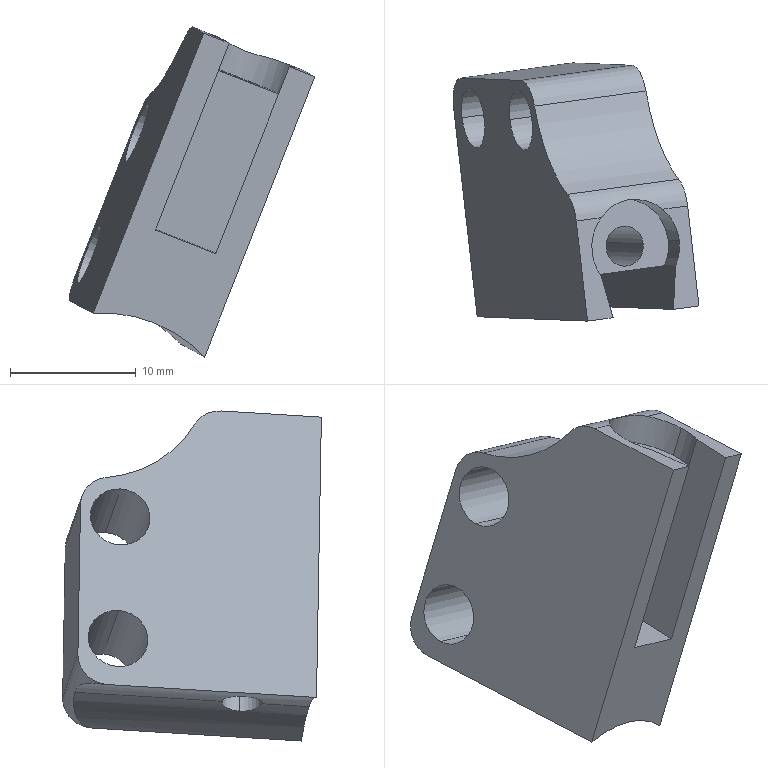Part | SolidWorks | features SplitBody 1 | 1 solid | 26 faces | box 19.582 x 20.608 x 26.296 mm | volume 2916 mm3 | cylinder 15 | plane 11 | commonest cylinder face diameters 4.8 x7 7.52 x3 3.2 x2 22.4 x2 19.2 x1
STEP:
#1=CARTESIAN_POINT('',(550.829,303.4,-344.866));
#2=VERTEX_POINT('',#1);
#3=CARTESIAN_POINT('',(555.434,305.978,-345.474));
#4=VERTEX_POINT('',#3);
#5=CARTESIAN_POINT('',(550.829,303.4,-344.866));
#6=CARTESIAN_POINT('',(550.801,303.644,-344.851));
#7=CARTESIAN_POINT('',(550.865,303.886,-344.83));
#8=CARTESIAN_POINT('',(551.105,304.312,-344.791));
#9=CARTESIAN_POINT('',(551.273,304.49,-344.775));
#10=CARTESIAN_POINT('',(551.646,304.799,-344.757));
#11=CARTESIAN_POINT('',(551.85,304.928,-344.755));
#12=CARTESIAN_POINT('',(552.277,305.154,-344.769));
#13=CARTESIAN_POINT('',(552.499,305.251,-344.784));
#14=CARTESIAN_POINT('',(553.17,305.506,-344.854));
#15=CARTESIAN_POINT('',(553.626,305.632,-344.933));
#16=CARTESIAN_POINT('',(554.544,305.84,-345.158));
#17=CARTESIAN_POINT('',(554.994,305.918,-345.302));
#18=CARTESIAN_POINT('',(555.434,305.978,-345.474));
#19=B_SPLINE_CURVE_WITH_KNOTS('',3,(#5,#6,#7,#8,#9,#10,#11,#12,#13,#14,#15,#16,#17,#18),.UNSPECIFIED.,.F.,.F.,(4,2,2,2,2,2,4),(0.,0.0007263,0.001453,0.002179,0.002905,0.004358,0.00581),.UNSPECIFIED.);
#20=EDGE_CURVE('',#2,#4,#19,.T.);
#21=ORIENTED_EDGE('',*,*,#20,.T.);
#22=CARTESIAN_POINT('',(556.757,294.247,-346.199));
#23=VERTEX_POINT('',#22);
#24=CARTESIAN_POINT('',(555.39,306.37,-345.45));
#25=DIRECTION('',(0.1119,-0.9918,-0.06132));
#26=VECTOR('',#25,1000.);
#27=LINE('',#24,#26);
#28=EDGE_CURVE('',#4,#23,#27,.T.);
#29=ORIENTED_EDGE('',*,*,#28,.T.);
#30=CARTESIAN_POINT('',(555.416,292.46,-345.826));
#31=VERTEX_POINT('',#30);
#32=CARTESIAN_POINT('',(555.416,292.46,-345.826));
#33=CARTESIAN_POINT('',(555.405,292.565,-345.819));
#34=CARTESIAN_POINT('',(555.403,292.669,-345.815));
#35=CARTESIAN_POINT('',(555.42,292.877,-345.812));
#36=CARTESIAN_POINT('',(555.439,292.982,-345.813));
#37=CARTESIAN_POINT('',(555.495,293.184,-345.82));
#38=CARTESIAN_POINT('',(555.533,293.282,-345.826));
#39=CARTESIAN_POINT('',(555.626,293.468,-345.845));
#40=CARTESIAN_POINT('',(555.682,293.558,-345.857));
#41=CARTESIAN_POINT('',(555.869,293.805,-345.903));
#42=CARTESIAN_POINT('',(556.026,293.946,-345.946));
#43=CARTESIAN_POINT('',(556.372,294.153,-346.056));
#44=CARTESIAN_POINT('',(556.564,294.221,-346.124));
#45=CARTESIAN_POINT('',(556.757,294.247,-346.199));
#46=B_SPLINE_CURVE_WITH_KNOTS('',3,(#32,#33,#34,#35,#36,#37,#38,#39,#40,#41,#42,#43,#44,#45),.UNSPECIFIED.,.F.,.F.,(4,2,2,2,2,2,4),(0.,0.0003131,0.0006262,0.0009394,0.001252,0.001879,0.002505),.UNSPECIFIED.);
#47=EDGE_CURVE('',#31,#23,#46,.T.);
#48=ORIENTED_EDGE('',*,*,#47,.F.);
#49=CARTESIAN_POINT('',(557.115,291.073,-346.396));
#50=VERTEX_POINT('',#49);
#51=CARTESIAN_POINT('',(557.115,291.073,-346.396));
#52=CARTESIAN_POINT('',(557.018,291.06,-346.357));
#53=CARTESIAN_POINT('',(556.92,291.057,-346.32));
#54=CARTESIAN_POINT('',(556.724,291.072,-346.249));
#55=CARTESIAN_POINT('',(556.625,291.09,-346.215));
#56=CARTESIAN_POINT('',(556.434,291.145,-346.15));
#57=CARTESIAN_POINT('',(556.341,291.182,-346.119));
#58=CARTESIAN_POINT('',(556.163,291.275,-346.062));
#59=CARTESIAN_POINT('',(556.076,291.332,-346.035));
#60=CARTESIAN_POINT('',(555.839,291.523,-345.963));
#61=CARTESIAN_POINT('',(555.704,291.685,-345.923));
#62=CARTESIAN_POINT('',(555.505,292.047,-345.861));
#63=CARTESIAN_POINT('',(555.44,292.25,-345.839));
#64=CARTESIAN_POINT('',(555.416,292.46,-345.826));
#65=B_SPLINE_CURVE_WITH_KNOTS('',3,(#51,#52,#53,#54,#55,#56,#57,#58,#59,#60,#61,#62,#63,#64),.UNSPECIFIED.,.F.,.F.,(4,2,2,2,2,2,4),(0.007514,0.007826,0.008139,0.008452,0.008765,0.009391,0.01002),.UNSPECIFIED.);
#66=EDGE_CURVE('',#50,#31,#65,.T.);
#67=ORIENTED_EDGE('',*,*,#66,.F.);
#68=CARTESIAN_POINT('',(557.538,287.327,-346.627));
#69=VERTEX_POINT('',#68);
#70=CARTESIAN_POINT('',(555.39,306.37,-345.45));
#71=DIRECTION('',(0.1119,-0.9918,-0.06132));
#72=VECTOR('',#71,1000.);
#73=LINE('',#70,#72);
#74=EDGE_CURVE('',#50,#69,#73,.T.);
#75=ORIENTED_EDGE('',*,*,#74,.T.);
#76=CARTESIAN_POINT('',(552.708,286.737,-345.897));
#77=VERTEX_POINT('',#76);
#78=CARTESIAN_POINT('',(553.434,287.509,-357.046));
#79=DIRECTION('',(0.1119,-0.9918,-0.06132));
#80=DIRECTION('',(0.3665,-0.01618,0.9303));
#81=AXIS2_PLACEMENT_3D('',#78,#79,#80);
#82=CIRCLE('',#81,11.2);
#83=EDGE_CURVE('',#69,#77,#82,.T.);
#84=ORIENTED_EDGE('',*,*,#83,.T.);
#85=CARTESIAN_POINT('',(552.708,286.737,-345.897));
#86=DIRECTION('',(0.1119,-0.9918,-0.06132));
#87=VECTOR('',#86,1000.);
#88=LINE('',#85,#87);
#89=EDGE_CURVE('',#2,#77,#88,.T.);
#90=ORIENTED_EDGE('',*,*,#89,.F.);
#91=EDGE_LOOP('',(#21,#29,#48,#67,#75,#84,#90));
#92=FACE_OUTER_BOUND('',#91,.T.);
#93=CARTESIAN_POINT('',(551.286,306.552,-355.869));
#94=DIRECTION('',(0.1119,-0.9918,-0.06132));
#95=DIRECTION('',(0.3665,-0.01618,0.9303));
#96=AXIS2_PLACEMENT_3D('',#93,#94,#95);
#97=CYLINDRICAL_SURFACE('',#96,11.2);
#98=ADVANCED_FACE('',(#92),#97,.F.);
#99=CARTESIAN_POINT('',(567.929,292.804,-328.568));
#100=VERTEX_POINT('',#99);
#101=CARTESIAN_POINT('',(560.983,291.852,-325.849));
#102=VERTEX_POINT('',#101);
#103=CARTESIAN_POINT('',(564.456,292.328,-327.208));
#104=DIRECTION('',(0.3665,-0.01618,0.9303));
#105=DIRECTION('',(-0.9237,-0.1265,0.3616));
#106=AXIS2_PLACEMENT_3D('',#103,#104,#105);
#107=CIRCLE('',#106,3.76);
#108=EDGE_CURVE('',#100,#102,#107,.T.);
#109=ORIENTED_EDGE('',*,*,#108,.F.);
#110=CARTESIAN_POINT('',(568.808,292.765,-326.335));
#111=VERTEX_POINT('',#110);
#112=CARTESIAN_POINT('',(567.929,292.804,-328.568));
#113=DIRECTION('',(0.3665,-0.01618,0.9303));
#114=VECTOR('',#113,1000.);
#115=LINE('',#112,#114);
#116=EDGE_CURVE('',#100,#111,#115,.T.);
#117=ORIENTED_EDGE('',*,*,#116,.T.);
#118=CARTESIAN_POINT('',(567.494,295.262,-325.774));
#119=VERTEX_POINT('',#118);
#120=CARTESIAN_POINT('',(565.335,292.289,-324.976));
#121=DIRECTION('',(0.3665,-0.01618,0.9303));
#122=DIRECTION('',(-0.9237,-0.1265,0.3616));
#123=AXIS2_PLACEMENT_3D('',#120,#121,#122);
#124=CIRCLE('',#123,3.76);
#125=EDGE_CURVE('',#111,#119,#124,.T.);
#126=ORIENTED_EDGE('',*,*,#125,.T.);
#127=CARTESIAN_POINT('',(562.581,294.589,-323.851));
#128=VERTEX_POINT('',#127);
#129=CARTESIAN_POINT('',(567.494,295.262,-325.774));
#130=CARTESIAN_POINT('',(567.311,295.416,-325.7));
#131=CARTESIAN_POINT('',(567.111,295.546,-325.639));
#132=CARTESIAN_POINT('',(566.685,295.765,-325.526));
#133=CARTESIAN_POINT('',(566.456,295.854,-325.472));
#134=CARTESIAN_POINT('',(565.992,295.984,-325.36));
#135=CARTESIAN_POINT('',(565.756,296.026,-325.301));
#136=CARTESIAN_POINT('',(565.281,296.061,-325.163));
#137=CARTESIAN_POINT('',(565.044,296.054,-325.083));
#138=CARTESIAN_POINT('',(564.59,295.992,-324.906));
#139=CARTESIAN_POINT('',(564.37,295.937,-324.806));
#140=CARTESIAN_POINT('',(563.948,295.778,-324.593));
#141=CARTESIAN_POINT('',(563.752,295.677,-324.483));
#142=CARTESIAN_POINT('',(563.38,295.433,-324.268));
#143=CARTESIAN_POINT('',(563.203,295.289,-324.162));
#144=CARTESIAN_POINT('',(562.877,294.966,-323.981));
#145=CARTESIAN_POINT('',(562.725,294.787,-323.904));
#146=CARTESIAN_POINT('',(562.581,294.589,-323.851));
#147=B_SPLINE_CURVE_WITH_KNOTS('',3,(#129,#130,#131,#132,#133,#134,#135,#136,#137,#138,#139,#140,#141,#142,#143,#144,#145,#146),.UNSPECIFIED.,.F.,.F.,(4,2,2,2,2,2,2,2,4),(0.,0.000738,0.001476,0.002214,0.002952,0.00369,0.004428,0.005166,0.005904),.UNSPECIFIED.);
#148=EDGE_CURVE('',#119,#128,#147,.T.);
#149=ORIENTED_EDGE('',*,*,#148,.T.);
#150=CARTESIAN_POINT('',(561.862,291.814,-323.616));
#151=VERTEX_POINT('',#150);
#152=CARTESIAN_POINT('',(565.335,292.289,-324.976));
#153=DIRECTION('',(0.3665,-0.01618,0.9303));
#154=DIRECTION('',(-0.9237,-0.1265,0.3616));
#155=AXIS2_PLACEMENT_3D('',#152,#153,#154);
#156=CIRCLE('',#155,3.76);
#157=EDGE_CURVE('',#128,#151,#156,.T.);
#158=ORIENTED_EDGE('',*,*,#157,.T.);
#159=CARTESIAN_POINT('',(560.983,291.852,-325.849));
#160=DIRECTION('',(0.3665,-0.01618,0.9303));
#161=VECTOR('',#160,1000.);
#162=LINE('',#159,#161);
#163=EDGE_CURVE('',#102,#151,#162,.T.);
#164=ORIENTED_EDGE('',*,*,#163,.F.);
#165=EDGE_LOOP('',(#109,#117,#126,#149,#158,#164));
#166=FACE_OUTER_BOUND('',#165,.T.);
#167=CARTESIAN_POINT('',(564.456,292.328,-327.208));
#168=DIRECTION('',(0.3665,-0.01618,0.9303));
#169=DIRECTION('',(-0.9237,-0.1265,0.3616));
#170=AXIS2_PLACEMENT_3D('',#167,#168,#169);
#171=CYLINDRICAL_SURFACE('',#170,3.76);
#172=ADVANCED_FACE('',(#166),#171,.F.);
#173=CARTESIAN_POINT('',(561.721,289.965,-326.172));
#174=VERTEX_POINT('',#173);
#175=CARTESIAN_POINT('',(564.456,292.328,-327.208));
#176=DIRECTION('',(0.3665,-0.01618,0.9303));
#177=DIRECTION('',(-0.9237,-0.1265,0.3616));
#178=AXIS2_PLACEMENT_3D('',#175,#176,#177);
#179=CIRCLE('',#178,3.76);
#180=EDGE_CURVE('',#102,#174,#179,.T.);
#181=ORIENTED_EDGE('',*,*,#180,.F.);
#182=ORIENTED_EDGE('',*,*,#163,.T.);
#183=CARTESIAN_POINT('',(562.6,289.926,-323.94));
#184=VERTEX_POINT('',#183);
#185=CARTESIAN_POINT('',(565.335,292.289,-324.976));
#186=DIRECTION('',(0.3665,-0.01618,0.9303));
#187=DIRECTION('',(-0.9237,-0.1265,0.3616));
#188=AXIS2_PLACEMENT_3D('',#185,#186,#187);
#189=CIRCLE('',#188,3.76);
#190=EDGE_CURVE('',#151,#184,#189,.T.);
#191=ORIENTED_EDGE('',*,*,#190,.T.);
#192=CARTESIAN_POINT('',(561.721,289.965,-326.172));
#193=DIRECTION('',(0.3665,-0.01618,0.9303));
#194=VECTOR('',#193,1000.);
#195=LINE('',#192,#194);
#196=EDGE_CURVE('',#174,#184,#195,.T.);
#197=ORIENTED_EDGE('',*,*,#196,.F.);
#198=EDGE_LOOP('',(#181,#182,#191,#197));
#199=FACE_OUTER_BOUND('',#198,.T.);
#200=CARTESIAN_POINT('',(564.456,292.328,-327.208));
#201=DIRECTION('',(0.3665,-0.01618,0.9303));
#202=DIRECTION('',(-0.9237,-0.1265,0.3616));
#203=AXIS2_PLACEMENT_3D('',#200,#201,#202);
#204=CYLINDRICAL_SURFACE('',#203,3.76);
#205=ADVANCED_FACE('',(#199),#204,.F.);
#206=CARTESIAN_POINT('',(553.264,302.503,-338.962));
#207=VERTEX_POINT('',#206);
#208=CARTESIAN_POINT('',(551.505,302.581,-343.427));
#209=VERTEX_POINT('',#208);
#210=CARTESIAN_POINT('',(552.384,302.542,-341.194));
#211=DIRECTION('',(-0.9237,-0.1265,0.3616));
#212=DIRECTION('',(-0.3665,0.01618,-0.9303));
#213=AXIS2_PLACEMENT_3D('',#210,#211,#212);
#214=CIRCLE('',#213,2.4);
#215=EDGE_CURVE('',#207,#209,#214,.T.);
#216=ORIENTED_EDGE('',*,*,#215,.T.);
#217=CARTESIAN_POINT('',(560.372,303.796,-346.899));
#218=VERTEX_POINT('',#217);
#219=CARTESIAN_POINT('',(551.505,302.581,-343.427));
#220=DIRECTION('',(0.9237,0.1265,-0.3616));
#221=VECTOR('',#220,1000.);
#222=LINE('',#219,#221);
#223=EDGE_CURVE('',#209,#218,#222,.T.);
#224=ORIENTED_EDGE('',*,*,#223,.T.);
#225=CARTESIAN_POINT('',(562.131,303.718,-342.433));
#226=VERTEX_POINT('',#225);
#227=CARTESIAN_POINT('',(561.252,303.757,-344.666));
#228=DIRECTION('',(-0.9237,-0.1265,0.3616));
#229=DIRECTION('',(-0.3665,0.01618,-0.9303));
#230=AXIS2_PLACEMENT_3D('',#227,#228,#229);
#231=CIRCLE('',#230,2.4);
#232=EDGE_CURVE('',#226,#218,#231,.T.);
#233=ORIENTED_EDGE('',*,*,#232,.F.);
#234=CARTESIAN_POINT('',(553.264,302.503,-338.962));
#235=DIRECTION('',(0.9237,0.1265,-0.3616));
#236=VECTOR('',#235,1000.);
#237=LINE('',#234,#236);
#238=EDGE_CURVE('',#207,#226,#237,.T.);
#239=ORIENTED_EDGE('',*,*,#238,.F.);
#240=EDGE_LOOP('',(#216,#224,#233,#239));
#241=FACE_OUTER_BOUND('',#240,.T.);
#242=CARTESIAN_POINT('',(552.384,302.542,-341.194));
#243=DIRECTION('',(0.9237,0.1265,-0.3616));
#244=DIRECTION('',(0.3665,-0.01618,0.9303));
#245=AXIS2_PLACEMENT_3D('',#242,#243,#244);
#246=CYLINDRICAL_SURFACE('',#245,2.4);
#247=ADVANCED_FACE('',(#241),#246,.F.);
#248=CARTESIAN_POINT('',(557.075,302.335,-329.287));
#249=VERTEX_POINT('',#248);
#250=CARTESIAN_POINT('',(555.316,302.412,-333.752));
#251=VERTEX_POINT('',#250);
#252=CARTESIAN_POINT('',(556.195,302.374,-331.519));
#253=DIRECTION('',(-0.9237,-0.1265,0.3616));
#254=DIRECTION('',(-0.3665,0.01618,-0.9303));
#255=AXIS2_PLACEMENT_3D('',#252,#253,#254);
#256=CIRCLE('',#255,2.4);
#257=EDGE_CURVE('',#249,#251,#256,.T.);
#258=ORIENTED_EDGE('',*,*,#257,.T.);
#259=CARTESIAN_POINT('',(564.183,303.627,-337.224));
#260=VERTEX_POINT('',#259);
#261=CARTESIAN_POINT('',(555.316,302.412,-333.752));
#262=DIRECTION('',(0.9237,0.1265,-0.3616));
#263=VECTOR('',#262,1000.);
#264=LINE('',#261,#263);
#265=EDGE_CURVE('',#251,#260,#264,.T.);
#266=ORIENTED_EDGE('',*,*,#265,.T.);
#267=CARTESIAN_POINT('',(565.942,303.55,-332.758));
#268=VERTEX_POINT('',#267);
#269=CARTESIAN_POINT('',(565.063,303.588,-334.991));
#270=DIRECTION('',(-0.9237,-0.1265,0.3616));
#271=DIRECTION('',(-0.3665,0.01618,-0.9303));
#272=AXIS2_PLACEMENT_3D('',#269,#270,#271);
#273=CIRCLE('',#272,2.4);
#274=EDGE_CURVE('',#268,#260,#273,.T.);
#275=ORIENTED_EDGE('',*,*,#274,.F.);
#276=CARTESIAN_POINT('',(557.075,302.335,-329.287));
#277=DIRECTION('',(0.9237,0.1265,-0.3616));
#278=VECTOR('',#277,1000.);
#279=LINE('',#276,#278);
#280=EDGE_CURVE('',#249,#268,#279,.T.);
#281=ORIENTED_EDGE('',*,*,#280,.F.);
#282=EDGE_LOOP('',(#258,#266,#275,#281));
#283=FACE_OUTER_BOUND('',#282,.T.);
#284=CARTESIAN_POINT('',(556.195,302.374,-331.519));
#285=DIRECTION('',(0.9237,0.1265,-0.3616));
#286=DIRECTION('',(0.3665,-0.01618,0.9303));
#287=AXIS2_PLACEMENT_3D('',#284,#285,#286);
#288=CYLINDRICAL_SURFACE('',#287,2.4);
#289=ADVANCED_FACE('',(#283),#288,.F.);
#290=ORIENTED_EDGE('',*,*,#47,.T.);
#291=CARTESIAN_POINT('',(558.372,292.865,-346.983));
#292=VERTEX_POINT('',#291);
#293=CARTESIAN_POINT('',(556.757,294.247,-346.199));
#294=CARTESIAN_POINT('',(556.854,294.261,-346.237));
#295=CARTESIAN_POINT('',(556.953,294.264,-346.278));
#296=CARTESIAN_POINT('',(557.145,294.249,-346.36));
#297=CARTESIAN_POINT('',(557.239,294.232,-346.401));
#298=CARTESIAN_POINT('',(557.423,294.177,-346.486));
#299=CARTESIAN_POINT('',(557.512,294.139,-346.529));
#300=CARTESIAN_POINT('',(557.68,294.046,-346.612));
#301=CARTESIAN_POINT('',(557.76,293.991,-346.652));
#302=CARTESIAN_POINT('',(557.909,293.862,-346.729));
#303=CARTESIAN_POINT('',(557.976,293.791,-346.765));
#304=CARTESIAN_POINT('',(558.097,293.634,-346.83));
#305=CARTESIAN_POINT('',(558.151,293.547,-346.86));
#306=CARTESIAN_POINT('',(558.243,293.366,-346.911));
#307=CARTESIAN_POINT('',(558.281,293.271,-346.932));
#308=CARTESIAN_POINT('',(558.34,293.072,-346.965));
#309=CARTESIAN_POINT('',(558.361,292.968,-346.977));
#310=CARTESIAN_POINT('',(558.372,292.865,-346.983));
#311=B_SPLINE_CURVE_WITH_KNOTS('',3,(#293,#294,#295,#296,#297,#298,#299,#300,#301,#302,#303,#304,#305,#306,#307,#308,#309,#310),.UNSPECIFIED.,.F.,.F.,(4,2,2,2,2,2,2,2,4),(0.002505,0.002818,0.003131,0.003444,0.003757,0.00407,0.004383,0.004696,0.005009),.UNSPECIFIED.);
#312=EDGE_CURVE('',#23,#292,#311,.T.);
#313=ORIENTED_EDGE('',*,*,#312,.T.);
#314=CARTESIAN_POINT('',(565.934,292.531,-327.787));
#315=VERTEX_POINT('',#314);
#316=CARTESIAN_POINT('',(558.018,292.88,-347.881));
#317=DIRECTION('',(0.3665,-0.01618,0.9303));
#318=VECTOR('',#317,1000.);
#319=LINE('',#316,#318);
#320=EDGE_CURVE('',#292,#315,#319,.T.);
#321=ORIENTED_EDGE('',*,*,#320,.T.);
#322=CARTESIAN_POINT('',(562.978,292.126,-326.63));
#323=VERTEX_POINT('',#322);
#324=CARTESIAN_POINT('',(564.456,292.328,-327.208));
#325=DIRECTION('',(0.3665,-0.01618,0.9303));
#326=DIRECTION('',(-0.9237,-0.1265,0.3616));
#327=AXIS2_PLACEMENT_3D('',#324,#325,#326);
#328=CIRCLE('',#327,1.6);
#329=EDGE_CURVE('',#315,#323,#328,.T.);
#330=ORIENTED_EDGE('',*,*,#329,.T.);
#331=CARTESIAN_POINT('',(555.063,292.475,-346.724));
#332=DIRECTION('',(0.3665,-0.01618,0.9303));
#333=VECTOR('',#332,1000.);
#334=LINE('',#331,#333);
#335=EDGE_CURVE('',#31,#323,#334,.T.);
#336=ORIENTED_EDGE('',*,*,#335,.F.);
#337=EDGE_LOOP('',(#290,#313,#321,#330,#336));
#338=FACE_OUTER_BOUND('',#337,.T.);
#339=CARTESIAN_POINT('',(556.54,292.678,-347.303));
#340=DIRECTION('',(0.3665,-0.01618,0.9303));
#341=DIRECTION('',(-0.9237,-0.1265,0.3616));
#342=AXIS2_PLACEMENT_3D('',#339,#340,#341);
#343=CYLINDRICAL_SURFACE('',#342,1.6);
#344=ADVANCED_FACE('',(#338),#343,.F.);
#345=CARTESIAN_POINT('',(563.535,286.627,-324.365));
#346=VERTEX_POINT('',#345);
#347=CARTESIAN_POINT('',(561.099,295.223,-323.256));
#348=DIRECTION('',(-0.2706,0.9548,0.1232));
#349=VECTOR('',#348,1000.);
#350=LINE('',#347,#349);
#351=EDGE_CURVE('',#346,#184,#350,.T.);
#352=ORIENTED_EDGE('',*,*,#351,.T.);
#353=ORIENTED_EDGE('',*,*,#190,.F.);
#354=ORIENTED_EDGE('',*,*,#157,.F.);
#355=CARTESIAN_POINT('',(560.604,294.318,-323.077));
#356=VERTEX_POINT('',#355);
#357=CARTESIAN_POINT('',(560.604,294.318,-323.077));
#358=DIRECTION('',(-0.9237,-0.1265,0.3616));
#359=VECTOR('',#358,1000.);
#360=LINE('',#357,#359);
#361=EDGE_CURVE('',#128,#356,#360,.T.);
#362=ORIENTED_EDGE('',*,*,#361,.T.);
#363=CARTESIAN_POINT('',(561.503,286.349,-323.57));
#364=VERTEX_POINT('',#363);
#365=CARTESIAN_POINT('',(561.503,286.349,-323.57));
#366=DIRECTION('',(-0.1119,0.9918,0.06132));
#367=VECTOR('',#366,1000.);
#368=LINE('',#365,#367);
#369=EDGE_CURVE('',#364,#356,#368,.T.);
#370=ORIENTED_EDGE('',*,*,#369,.F.);
#371=CARTESIAN_POINT('',(561.503,286.349,-323.57));
#372=DIRECTION('',(0.9237,0.1265,-0.3616));
#373=VECTOR('',#372,1000.);
#374=LINE('',#371,#373);
#375=EDGE_CURVE('',#364,#346,#374,.T.);
#376=ORIENTED_EDGE('',*,*,#375,.T.);
#377=EDGE_LOOP('',(#352,#353,#354,#362,#370,#376));
#378=FACE_OUTER_BOUND('',#377,.T.);
#379=CARTESIAN_POINT('',(561.503,286.349,-323.57));
#380=DIRECTION('',(-0.3665,0.01618,-0.9303));
#381=DIRECTION('',(0.1119,-0.9918,-0.06132));
#382=AXIS2_PLACEMENT_3D('',#379,#380,#381);
#383=PLANE('',#382);
#384=ADVANCED_FACE('',(#378),#383,.F.);
#385=ORIENTED_EDGE('',*,*,#320,.F.);
#386=CARTESIAN_POINT('',(558.372,292.865,-346.983));
#387=CARTESIAN_POINT('',(558.396,292.657,-346.996));
#388=CARTESIAN_POINT('',(558.383,292.443,-346.988));
#389=CARTESIAN_POINT('',(558.286,292.04,-346.934));
#390=CARTESIAN_POINT('',(558.202,291.848,-346.888));
#391=CARTESIAN_POINT('',(558.03,291.6,-346.8));
#392=CARTESIAN_POINT('',(557.965,291.523,-346.768));
#393=CARTESIAN_POINT('',(557.822,291.385,-346.699));
#394=CARTESIAN_POINT('',(557.745,291.325,-346.663));
#395=CARTESIAN_POINT('',(557.579,291.22,-346.588));
#396=CARTESIAN_POINT('',(557.49,291.177,-346.549));
#397=CARTESIAN_POINT('',(557.308,291.11,-346.472));
#398=CARTESIAN_POINT('',(557.213,291.087,-346.434));
#399=CARTESIAN_POINT('',(557.115,291.073,-346.396));
#400=B_SPLINE_CURVE_WITH_KNOTS('',3,(#386,#387,#388,#389,#390,#391,#392,#393,#394,#395,#396,#397,#398,#399),.UNSPECIFIED.,.F.,.F.,(4,2,2,2,2,2,4),(0.005009,0.005635,0.006261,0.006574,0.006887,0.0072,0.007514),.UNSPECIFIED.);
#401=EDGE_CURVE('',#292,#50,#400,.T.);
#402=ORIENTED_EDGE('',*,*,#401,.T.);
#403=ORIENTED_EDGE('',*,*,#66,.T.);
#404=ORIENTED_EDGE('',*,*,#335,.T.);
#405=CARTESIAN_POINT('',(564.456,292.328,-327.208));
#406=DIRECTION('',(0.3665,-0.01618,0.9303));
#407=DIRECTION('',(-0.9237,-0.1265,0.3616));
#408=AXIS2_PLACEMENT_3D('',#405,#406,#407);
#409=CIRCLE('',#408,1.6);
#410=EDGE_CURVE('',#323,#315,#409,.T.);
#411=ORIENTED_EDGE('',*,*,#410,.T.);
#412=EDGE_LOOP('',(#385,#402,#403,#404,#411));
#413=FACE_OUTER_BOUND('',#412,.T.);
#414=CARTESIAN_POINT('',(556.54,292.678,-347.303));
#415=DIRECTION('',(0.3665,-0.01618,0.9303));
#416=DIRECTION('',(-0.9237,-0.1265,0.3616));
#417=AXIS2_PLACEMENT_3D('',#414,#415,#416);
#418=CYLINDRICAL_SURFACE('',#417,1.6);
#419=ADVANCED_FACE('',(#413),#418,.F.);
#420=CARTESIAN_POINT('',(562.649,290.995,-341.139));
#421=VERTEX_POINT('',#420);
#422=CARTESIAN_POINT('',(567.632,290.775,-328.487));
#423=VERTEX_POINT('',#422);
#424=CARTESIAN_POINT('',(562.649,290.995,-341.139));
#425=DIRECTION('',(0.3665,-0.01618,0.9303));
#426=VECTOR('',#425,1000.);
#427=LINE('',#424,#426);
#428=EDGE_CURVE('',#421,#423,#427,.T.);
#429=ORIENTED_EDGE('',*,*,#428,.T.);
#430=CARTESIAN_POINT('',(564.677,290.37,-327.329));
#431=DIRECTION('',(0.9237,0.1265,-0.3616));
#432=VECTOR('',#431,1000.);
#433=LINE('',#430,#432);
#434=EDGE_CURVE('',#174,#423,#433,.T.);
#435=ORIENTED_EDGE('',*,*,#434,.F.);
#436=CARTESIAN_POINT('',(556.737,290.185,-338.824));
#437=VERTEX_POINT('',#436);
#438=CARTESIAN_POINT('',(556.737,290.185,-338.824));
#439=DIRECTION('',(0.3665,-0.01618,0.9303));
#440=VECTOR('',#439,1000.);
#441=LINE('',#438,#440);
#442=EDGE_CURVE('',#437,#174,#441,.T.);
#443=ORIENTED_EDGE('',*,*,#442,.F.);
#444=CARTESIAN_POINT('',(559.693,290.59,-339.982));
#445=DIRECTION('',(0.9237,0.1265,-0.3616));
#446=VECTOR('',#445,1000.);
#447=LINE('',#444,#446);
#448=EDGE_CURVE('',#437,#421,#447,.T.);
#449=ORIENTED_EDGE('',*,*,#448,.T.);
#450=EDGE_LOOP('',(#429,#435,#443,#449));
#451=FACE_OUTER_BOUND('',#450,.T.);
#452=CARTESIAN_POINT('',(559.693,290.59,-339.982));
#453=DIRECTION('',(0.1119,-0.9918,-0.06132));
#454=DIRECTION('',(0.9237,0.1265,-0.3616));
#455=AXIS2_PLACEMENT_3D('',#452,#453,#454);
#456=PLANE('',#455);
#457=ADVANCED_FACE('',(#451),#456,.T.);
#458=CARTESIAN_POINT('',(569.472,295.533,-326.549));
#459=VERTEX_POINT('',#458);
#460=CARTESIAN_POINT('',(560.604,294.318,-323.077));
#461=DIRECTION('',(-0.9237,-0.1265,0.3616));
#462=VECTOR('',#461,1000.);
#463=LINE('',#460,#462);
#464=EDGE_CURVE('',#459,#119,#463,.T.);
#465=ORIENTED_EDGE('',*,*,#464,.T.);
#466=ORIENTED_EDGE('',*,*,#125,.F.);
#467=CARTESIAN_POINT('',(568.512,290.736,-326.254));
#468=VERTEX_POINT('',#467);
#469=CARTESIAN_POINT('',(565.335,292.289,-324.976));
#470=DIRECTION('',(0.3665,-0.01618,0.9303));
#471=DIRECTION('',(-0.9237,-0.1265,0.3616));
#472=AXIS2_PLACEMENT_3D('',#469,#470,#471);
#473=CIRCLE('',#472,3.76);
#474=EDGE_CURVE('',#468,#111,#473,.T.);
#475=ORIENTED_EDGE('',*,*,#474,.F.);
#476=CARTESIAN_POINT('',(568.338,287.285,-326.246));
#477=VERTEX_POINT('',#476);
#478=CARTESIAN_POINT('',(568.791,296.277,-326.267));
#479=DIRECTION('',(-0.05022,-0.9987,0.002409));
#480=VECTOR('',#479,1000.);
#481=LINE('',#478,#480);
#482=EDGE_CURVE('',#468,#477,#481,.T.);
#483=ORIENTED_EDGE('',*,*,#482,.T.);
#484=CARTESIAN_POINT('',(570.371,287.564,-327.041));
#485=VERTEX_POINT('',#484);
#486=CARTESIAN_POINT('',(561.503,286.349,-323.57));
#487=DIRECTION('',(0.9237,0.1265,-0.3616));
#488=VECTOR('',#487,1000.);
#489=LINE('',#486,#488);
#490=EDGE_CURVE('',#477,#485,#489,.T.);
#491=ORIENTED_EDGE('',*,*,#490,.T.);
#492=CARTESIAN_POINT('',(570.371,287.564,-327.041));
#493=DIRECTION('',(-0.1119,0.9918,0.06132));
#494=VECTOR('',#493,1000.);
#495=LINE('',#492,#494);
#496=EDGE_CURVE('',#485,#459,#495,.T.);
#497=ORIENTED_EDGE('',*,*,#496,.T.);
#498=EDGE_LOOP('',(#465,#466,#475,#483,#491,#497));
#499=FACE_OUTER_BOUND('',#498,.T.);
#500=CARTESIAN_POINT('',(561.503,286.349,-323.57));
#501=DIRECTION('',(-0.3665,0.01618,-0.9303));
#502=DIRECTION('',(0.1119,-0.9918,-0.06132));
#503=AXIS2_PLACEMENT_3D('',#500,#501,#502);
#504=PLANE('',#503);
#505=ADVANCED_FACE('',(#499),#504,.F.);
#506=CARTESIAN_POINT('',(561.503,286.349,-323.57));
#507=DIRECTION('',(0.3665,-0.01618,0.9303));
#508=VECTOR('',#507,1000.);
#509=LINE('',#506,#508);
#510=EDGE_CURVE('',#77,#364,#509,.T.);
#511=ORIENTED_EDGE('',*,*,#510,.F.);
#512=ORIENTED_EDGE('',*,*,#83,.F.);
#513=CARTESIAN_POINT('',(561.576,287.952,-349.368));
#514=VERTEX_POINT('',#513);
#515=CARTESIAN_POINT('',(553.434,287.509,-357.046));
#516=DIRECTION('',(0.1119,-0.9918,-0.06132));
#517=DIRECTION('',(0.3665,-0.01618,0.9303));
#518=AXIS2_PLACEMENT_3D('',#515,#516,#517);
#519=CIRCLE('',#518,11.2);
#520=EDGE_CURVE('',#514,#69,#519,.T.);
#521=ORIENTED_EDGE('',*,*,#520,.F.);
#522=CARTESIAN_POINT('',(570.371,287.564,-327.041));
#523=DIRECTION('',(0.3665,-0.01618,0.9303));
#524=VECTOR('',#523,1000.);
#525=LINE('',#522,#524);
#526=EDGE_CURVE('',#514,#485,#525,.T.);
#527=ORIENTED_EDGE('',*,*,#526,.T.);
#528=ORIENTED_EDGE('',*,*,#490,.F.);
#529=CARTESIAN_POINT('',(562.475,287.544,-341.13));
#530=VERTEX_POINT('',#529);
#531=CARTESIAN_POINT('',(562.475,287.544,-341.13));
#532=DIRECTION('',(0.3665,-0.01618,0.9303));
#533=VECTOR('',#532,1000.);
#534=LINE('',#531,#533);
#535=EDGE_CURVE('',#530,#477,#534,.T.);
#536=ORIENTED_EDGE('',*,*,#535,.F.);
#537=CARTESIAN_POINT('',(557.672,286.886,-339.25));
#538=VERTEX_POINT('',#537);
#539=CARTESIAN_POINT('',(560.074,287.215,-340.19));
#540=DIRECTION('',(0.9237,0.1265,-0.3616));
#541=VECTOR('',#540,1000.);
#542=LINE('',#539,#541);
#543=EDGE_CURVE('',#538,#530,#542,.T.);
#544=ORIENTED_EDGE('',*,*,#543,.F.);
#545=CARTESIAN_POINT('',(557.672,286.886,-339.25));
#546=DIRECTION('',(0.3665,-0.01618,0.9303));
#547=VECTOR('',#546,1000.);
#548=LINE('',#545,#547);
#549=EDGE_CURVE('',#538,#346,#548,.T.);
#550=ORIENTED_EDGE('',*,*,#549,.T.);
#551=ORIENTED_EDGE('',*,*,#375,.F.);
#552=EDGE_LOOP('',(#511,#512,#521,#527,#528,#536,#544,#550,#551));
#553=FACE_OUTER_BOUND('',#552,.T.);
#554=CARTESIAN_POINT('',(561.503,286.349,-323.57));
#555=DIRECTION('',(-0.1119,0.9918,0.06132));
#556=DIRECTION('',(-0.3665,0.01618,-0.9303));
#557=AXIS2_PLACEMENT_3D('',#554,#555,#556);
#558=PLANE('',#557);
#559=ADVANCED_FACE('',(#553),#558,.F.);
#560=CARTESIAN_POINT('',(556.178,305.532,-330.459));
#561=VERTEX_POINT('',#560);
#562=CARTESIAN_POINT('',(551.44,305.742,-342.487));
#563=VERTEX_POINT('',#562);
#564=CARTESIAN_POINT('',(557.01,305.496,-328.346));
#565=DIRECTION('',(-0.3665,0.01618,-0.9303));
#566=VECTOR('',#565,1000.);
#567=LINE('',#564,#566);
#568=EDGE_CURVE('',#561,#563,#567,.T.);
#569=ORIENTED_EDGE('',*,*,#568,.T.);
#570=CARTESIAN_POINT('',(551.708,303.361,-342.634));
#571=DIRECTION('',(-0.9237,-0.1265,0.3616));
#572=DIRECTION('',(0.3665,-0.01618,0.9303));
#573=AXIS2_PLACEMENT_3D('',#570,#571,#572);
#574=CIRCLE('',#573,2.4);
#575=EDGE_CURVE('',#563,#2,#574,.T.);
#576=ORIENTED_EDGE('',*,*,#575,.T.);
#577=ORIENTED_EDGE('',*,*,#89,.T.);
#578=ORIENTED_EDGE('',*,*,#510,.T.);
#579=ORIENTED_EDGE('',*,*,#369,.T.);
#580=CARTESIAN_POINT('',(559.896,296.446,-324.14));
#581=VERTEX_POINT('',#580);
#582=CARTESIAN_POINT('',(559.725,294.357,-325.31));
#583=DIRECTION('',(-0.9237,-0.1265,0.3616));
#584=DIRECTION('',(0.3665,-0.01618,0.9303));
#585=AXIS2_PLACEMENT_3D('',#582,#583,#584);
#586=CIRCLE('',#585,2.4);
#587=EDGE_CURVE('',#356,#581,#586,.T.);
#588=ORIENTED_EDGE('',*,*,#587,.T.);
#589=CARTESIAN_POINT('',(557.274,303.482,-328.377));
#590=VERTEX_POINT('',#589);
#591=CARTESIAN_POINT('',(560.583,304.801,-319.463));
#592=DIRECTION('',(0.9237,0.1265,-0.3616));
#593=DIRECTION('',(0.3665,-0.01618,0.9303));
#594=AXIS2_PLACEMENT_3D('',#591,#592,#593);
#595=CIRCLE('',#594,9.6);
#596=EDGE_CURVE('',#581,#590,#595,.T.);
#597=ORIENTED_EDGE('',*,*,#596,.T.);
#598=CARTESIAN_POINT('',(556.446,303.152,-330.606));
#599=DIRECTION('',(-0.9237,-0.1265,0.3616));
#600=DIRECTION('',(0.3665,-0.01618,0.9303));
#601=AXIS2_PLACEMENT_3D('',#598,#599,#600);
#602=CIRCLE('',#601,2.4);
#603=EDGE_CURVE('',#590,#561,#602,.T.);
#604=ORIENTED_EDGE('',*,*,#603,.T.);
#605=EDGE_LOOP('',(#569,#576,#577,#578,#579,#588,#597,#604));
#606=FACE_OUTER_BOUND('',#605,.T.);
#607=ORIENTED_EDGE('',*,*,#257,.F.);
#608=CARTESIAN_POINT('',(556.195,302.374,-331.519));
#609=DIRECTION('',(-0.9237,-0.1265,0.3616));
#610=DIRECTION('',(-0.3665,0.01618,-0.9303));
#611=AXIS2_PLACEMENT_3D('',#608,#609,#610);
#612=CIRCLE('',#611,2.4);
#613=EDGE_CURVE('',#251,#249,#612,.T.);
#614=ORIENTED_EDGE('',*,*,#613,.F.);
#615=EDGE_LOOP('',(#607,#614));
#616=FACE_BOUND('',#615,.T.);
#617=ORIENTED_EDGE('',*,*,#215,.F.);
#618=CARTESIAN_POINT('',(552.384,302.542,-341.194));
#619=DIRECTION('',(-0.9237,-0.1265,0.3616));
#620=DIRECTION('',(-0.3665,0.01618,-0.9303));
#621=AXIS2_PLACEMENT_3D('',#618,#619,#620);
#622=CIRCLE('',#621,2.4);
#623=EDGE_CURVE('',#209,#207,#622,.T.);
#624=ORIENTED_EDGE('',*,*,#623,.F.);
#625=EDGE_LOOP('',(#617,#624));
#626=FACE_BOUND('',#625,.T.);
#627=CARTESIAN_POINT('',(560.583,304.801,-319.463));
#628=DIRECTION('',(0.9237,0.1265,-0.3616));
#629=DIRECTION('',(0.3665,-0.01618,0.9303));
#630=AXIS2_PLACEMENT_3D('',#627,#628,#629);
#631=PLANE('',#630);
#632=ADVANCED_FACE('',(#606,#616,#626),#631,.F.);
#633=ORIENTED_EDGE('',*,*,#274,.T.);
#634=CARTESIAN_POINT('',(565.063,303.588,-334.991));
#635=DIRECTION('',(-0.9237,-0.1265,0.3616));
#636=DIRECTION('',(-0.3665,0.01618,-0.9303));
#637=AXIS2_PLACEMENT_3D('',#634,#635,#636);
#638=CIRCLE('',#637,2.4);
#639=EDGE_CURVE('',#260,#268,#638,.T.);
#640=ORIENTED_EDGE('',*,*,#639,.T.);
#641=EDGE_LOOP('',(#633,#640));
#642=FACE_BOUND('',#641,.T.);
#643=CARTESIAN_POINT('',(559.696,304.615,-348.338));
#644=VERTEX_POINT('',#643);
#645=CARTESIAN_POINT('',(561.576,287.952,-349.368));
#646=DIRECTION('',(0.1119,-0.9918,-0.06132));
#647=VECTOR('',#646,1000.);
#648=LINE('',#645,#647);
#649=EDGE_CURVE('',#644,#514,#648,.T.);
#650=ORIENTED_EDGE('',*,*,#649,.F.);
#651=CARTESIAN_POINT('',(560.307,306.956,-345.958));
#652=VERTEX_POINT('',#651);
#653=CARTESIAN_POINT('',(560.576,304.576,-346.106));
#654=DIRECTION('',(0.9237,0.1265,-0.3616));
#655=DIRECTION('',(0.3665,-0.01618,0.9303));
#656=AXIS2_PLACEMENT_3D('',#653,#654,#655);
#657=CIRCLE('',#656,2.4);
#658=EDGE_CURVE('',#644,#652,#657,.T.);
#659=ORIENTED_EDGE('',*,*,#658,.T.);
#660=CARTESIAN_POINT('',(565.045,306.747,-333.931));
#661=VERTEX_POINT('',#660);
#662=CARTESIAN_POINT('',(565.877,306.71,-331.818));
#663=DIRECTION('',(-0.3665,0.01618,-0.9303));
#664=VECTOR('',#663,1000.);
#665=LINE('',#662,#664);
#666=EDGE_CURVE('',#661,#652,#665,.T.);
#667=ORIENTED_EDGE('',*,*,#666,.F.);
#668=CARTESIAN_POINT('',(566.141,304.697,-331.849));
#669=VERTEX_POINT('',#668);
#670=CARTESIAN_POINT('',(565.314,304.367,-334.078));
#671=DIRECTION('',(0.9237,0.1265,-0.3616));
#672=DIRECTION('',(0.3665,-0.01618,0.9303));
#673=AXIS2_PLACEMENT_3D('',#670,#671,#672);
#674=CIRCLE('',#673,2.4);
#675=EDGE_CURVE('',#661,#669,#674,.T.);
#676=ORIENTED_EDGE('',*,*,#675,.T.);
#677=CARTESIAN_POINT('',(568.764,297.661,-327.612));
#678=VERTEX_POINT('',#677);
#679=CARTESIAN_POINT('',(569.45,306.016,-322.935));
#680=DIRECTION('',(0.9237,0.1265,-0.3616));
#681=DIRECTION('',(0.3665,-0.01618,0.9303));
#682=AXIS2_PLACEMENT_3D('',#679,#680,#681);
#683=CIRCLE('',#682,9.6);
#684=EDGE_CURVE('',#678,#669,#683,.T.);
#685=ORIENTED_EDGE('',*,*,#684,.F.);
#686=CARTESIAN_POINT('',(568.592,295.572,-328.781));
#687=DIRECTION('',(0.9237,0.1265,-0.3616));
#688=DIRECTION('',(0.3665,-0.01618,0.9303));
#689=AXIS2_PLACEMENT_3D('',#686,#687,#688);
#690=CIRCLE('',#689,2.4);
#691=EDGE_CURVE('',#678,#459,#690,.T.);
#692=ORIENTED_EDGE('',*,*,#691,.T.);
#693=ORIENTED_EDGE('',*,*,#496,.F.);
#694=ORIENTED_EDGE('',*,*,#526,.F.);
#695=EDGE_LOOP('',(#650,#659,#667,#676,#685,#692,#693,#694));
#696=FACE_OUTER_BOUND('',#695,.T.);
#697=ORIENTED_EDGE('',*,*,#232,.T.);
#698=CARTESIAN_POINT('',(561.252,303.757,-344.666));
#699=DIRECTION('',(-0.9237,-0.1265,0.3616));
#700=DIRECTION('',(-0.3665,0.01618,-0.9303));
#701=AXIS2_PLACEMENT_3D('',#698,#699,#700);
#702=CIRCLE('',#701,2.4);
#703=EDGE_CURVE('',#218,#226,#702,.T.);
#704=ORIENTED_EDGE('',*,*,#703,.T.);
#705=EDGE_LOOP('',(#697,#704));
#706=FACE_BOUND('',#705,.T.);
#707=CARTESIAN_POINT('',(569.45,306.016,-322.935));
#708=DIRECTION('',(0.9237,0.1265,-0.3616));
#709=DIRECTION('',(0.3665,-0.01618,0.9303));
#710=AXIS2_PLACEMENT_3D('',#707,#708,#709);
#711=PLANE('',#710);
#712=ADVANCED_FACE('',(#642,#696,#706),#711,.T.);
#713=ORIENTED_EDGE('',*,*,#684,.T.);
#714=CARTESIAN_POINT('',(557.274,303.482,-328.377));
#715=DIRECTION('',(-0.9237,-0.1265,0.3616));
#716=VECTOR('',#715,1000.);
#717=LINE('',#714,#716);
#718=EDGE_CURVE('',#669,#590,#717,.T.);
#719=ORIENTED_EDGE('',*,*,#718,.T.);
#720=ORIENTED_EDGE('',*,*,#596,.F.);
#721=CARTESIAN_POINT('',(559.896,296.446,-324.14));
#722=DIRECTION('',(0.9237,0.1265,-0.3616));
#723=VECTOR('',#722,1000.);
#724=LINE('',#721,#723);
#725=EDGE_CURVE('',#581,#678,#724,.T.);
#726=ORIENTED_EDGE('',*,*,#725,.T.);
#727=EDGE_LOOP('',(#713,#719,#720,#726));
#728=FACE_OUTER_BOUND('',#727,.T.);
#729=CARTESIAN_POINT('',(560.583,304.801,-319.463));
#730=DIRECTION('',(0.9237,0.1265,-0.3616));
#731=DIRECTION('',(0.3665,-0.01618,0.9303));
#732=AXIS2_PLACEMENT_3D('',#729,#730,#731);
#733=CYLINDRICAL_SURFACE('',#732,9.6);
#734=ADVANCED_FACE('',(#728),#733,.F.);
#735=ORIENTED_EDGE('',*,*,#666,.T.);
#736=CARTESIAN_POINT('',(551.44,305.742,-342.487));
#737=DIRECTION('',(-0.9237,-0.1265,0.3616));
#738=VECTOR('',#737,1000.);
#739=LINE('',#736,#738);
#740=EDGE_CURVE('',#652,#563,#739,.T.);
#741=ORIENTED_EDGE('',*,*,#740,.T.);
#742=ORIENTED_EDGE('',*,*,#568,.F.);
#743=CARTESIAN_POINT('',(556.178,305.532,-330.459));
#744=DIRECTION('',(0.9237,0.1265,-0.3616));
#745=VECTOR('',#744,1000.);
#746=LINE('',#743,#745);
#747=EDGE_CURVE('',#561,#661,#746,.T.);
#748=ORIENTED_EDGE('',*,*,#747,.T.);
#749=EDGE_LOOP('',(#735,#741,#742,#748));
#750=FACE_OUTER_BOUND('',#749,.T.);
#751=CARTESIAN_POINT('',(557.01,305.496,-328.346));
#752=DIRECTION('',(0.1119,-0.9918,-0.06132));
#753=DIRECTION('',(0.3665,-0.01618,0.9303));
#754=AXIS2_PLACEMENT_3D('',#751,#752,#753);
#755=PLANE('',#754);
#756=ADVANCED_FACE('',(#750),#755,.F.);
#757=ORIENTED_EDGE('',*,*,#265,.F.);
#758=ORIENTED_EDGE('',*,*,#613,.T.);
#759=ORIENTED_EDGE('',*,*,#280,.T.);
#760=ORIENTED_EDGE('',*,*,#639,.F.);
#761=EDGE_LOOP('',(#757,#758,#759,#760));
#762=FACE_OUTER_BOUND('',#761,.T.);
#763=CARTESIAN_POINT('',(556.195,302.374,-331.519));
#764=DIRECTION('',(0.9237,0.1265,-0.3616));
#765=DIRECTION('',(0.3665,-0.01618,0.9303));
#766=AXIS2_PLACEMENT_3D('',#763,#764,#765);
#767=CYLINDRICAL_SURFACE('',#766,2.4);
#768=ADVANCED_FACE('',(#762),#767,.F.);
#769=ORIENTED_EDGE('',*,*,#223,.F.);
#770=ORIENTED_EDGE('',*,*,#623,.T.);
#771=ORIENTED_EDGE('',*,*,#238,.T.);
#772=ORIENTED_EDGE('',*,*,#703,.F.);
#773=EDGE_LOOP('',(#769,#770,#771,#772));
#774=FACE_OUTER_BOUND('',#773,.T.);
#775=CARTESIAN_POINT('',(552.384,302.542,-341.194));
#776=DIRECTION('',(0.9237,0.1265,-0.3616));
#777=DIRECTION('',(0.3665,-0.01618,0.9303));
#778=AXIS2_PLACEMENT_3D('',#775,#776,#777);
#779=CYLINDRICAL_SURFACE('',#778,2.4);
#780=ADVANCED_FACE('',(#774),#779,.F.);
#781=ORIENTED_EDGE('',*,*,#20,.F.);
#782=ORIENTED_EDGE('',*,*,#575,.F.);
#783=ORIENTED_EDGE('',*,*,#740,.F.);
#784=ORIENTED_EDGE('',*,*,#658,.F.);
#785=CARTESIAN_POINT('',(555.434,305.978,-345.474));
#786=CARTESIAN_POINT('',(555.875,306.039,-345.646));
#787=CARTESIAN_POINT('',(556.306,306.081,-345.848));
#788=CARTESIAN_POINT('',(557.15,306.115,-346.312));
#789=CARTESIAN_POINT('',(557.559,306.108,-346.572));
#790=CARTESIAN_POINT('',(558.142,306.023,-346.994));
#791=CARTESIAN_POINT('',(558.331,305.983,-347.14));
#792=CARTESIAN_POINT('',(558.693,305.865,-347.435));
#793=CARTESIAN_POINT('',(558.866,305.788,-347.584));
#794=CARTESIAN_POINT('',(559.11,305.627,-347.803));
#795=CARTESIAN_POINT('',(559.187,305.567,-347.874));
#796=CARTESIAN_POINT('',(559.332,305.427,-348.009));
#797=CARTESIAN_POINT('',(559.401,305.348,-348.073));
#798=CARTESIAN_POINT('',(559.58,305.082,-348.241));
#799=CARTESIAN_POINT('',(559.669,304.858,-348.323));
#800=CARTESIAN_POINT('',(559.696,304.615,-348.338));
#801=B_SPLINE_CURVE_WITH_KNOTS('',3,(#785,#786,#787,#788,#789,#790,#791,#792,#793,#794,#795,#796,#797,#798,#799,#800),.UNSPECIFIED.,.F.,.F.,(4,2,2,2,2,2,2,4),(0.00581,0.007263,0.008716,0.009442,0.01017,0.01053,0.0109,0.01162),.UNSPECIFIED.);
#802=EDGE_CURVE('',#4,#644,#801,.T.);
#803=ORIENTED_EDGE('',*,*,#802,.F.);
#804=EDGE_LOOP('',(#781,#782,#783,#784,#803));
#805=FACE_OUTER_BOUND('',#804,.T.);
#806=CARTESIAN_POINT('',(551.708,303.361,-342.634));
#807=DIRECTION('',(0.9237,0.1265,-0.3616));
#808=DIRECTION('',(0.3665,-0.01618,0.9303));
#809=AXIS2_PLACEMENT_3D('',#806,#807,#808);
#810=CYLINDRICAL_SURFACE('',#809,2.4);
#811=ADVANCED_FACE('',(#805),#810,.T.);
#812=ORIENTED_EDGE('',*,*,#603,.F.);
#813=ORIENTED_EDGE('',*,*,#718,.F.);
#814=ORIENTED_EDGE('',*,*,#675,.F.);
#815=ORIENTED_EDGE('',*,*,#747,.F.);
#816=EDGE_LOOP('',(#812,#813,#814,#815));
#817=FACE_OUTER_BOUND('',#816,.T.);
#818=CARTESIAN_POINT('',(556.446,303.152,-330.606));
#819=DIRECTION('',(0.9237,0.1265,-0.3616));
#820=DIRECTION('',(0.3665,-0.01618,0.9303));
#821=AXIS2_PLACEMENT_3D('',#818,#819,#820);
#822=CYLINDRICAL_SURFACE('',#821,2.4);
#823=ADVANCED_FACE('',(#817),#822,.T.);
#824=ORIENTED_EDGE('',*,*,#148,.F.);
#825=ORIENTED_EDGE('',*,*,#464,.F.);
#826=ORIENTED_EDGE('',*,*,#691,.F.);
#827=ORIENTED_EDGE('',*,*,#725,.F.);
#828=ORIENTED_EDGE('',*,*,#587,.F.);
#829=ORIENTED_EDGE('',*,*,#361,.F.);
#830=EDGE_LOOP('',(#824,#825,#826,#827,#828,#829));
#831=FACE_OUTER_BOUND('',#830,.T.);
#832=CARTESIAN_POINT('',(559.725,294.357,-325.31));
#833=DIRECTION('',(0.9237,0.1265,-0.3616));
#834=DIRECTION('',(0.3665,-0.01618,0.9303));
#835=AXIS2_PLACEMENT_3D('',#832,#833,#834);
#836=CYLINDRICAL_SURFACE('',#835,2.4);
#837=ADVANCED_FACE('',(#831),#836,.T.);
#838=ORIENTED_EDGE('',*,*,#482,.F.);
#839=CARTESIAN_POINT('',(567.632,290.775,-328.487));
#840=DIRECTION('',(0.3665,-0.01618,0.9303));
#841=VECTOR('',#840,1000.);
#842=LINE('',#839,#841);
#843=EDGE_CURVE('',#423,#468,#842,.T.);
#844=ORIENTED_EDGE('',*,*,#843,.F.);
#845=ORIENTED_EDGE('',*,*,#428,.F.);
#846=CARTESIAN_POINT('',(562.927,296.536,-341.152));
#847=DIRECTION('',(-0.05022,-0.9987,0.002409));
#848=VECTOR('',#847,1000.);
#849=LINE('',#846,#848);
#850=EDGE_CURVE('',#421,#530,#849,.T.);
#851=ORIENTED_EDGE('',*,*,#850,.T.);
#852=ORIENTED_EDGE('',*,*,#535,.T.);
#853=EDGE_LOOP('',(#838,#844,#845,#851,#852));
#854=FACE_OUTER_BOUND('',#853,.T.);
#855=CARTESIAN_POINT('',(562.927,296.536,-341.152));
#856=DIRECTION('',(-0.9291,0.0476,0.3668));
#857=DIRECTION('',(-0.05022,-0.9987,0.002409));
#858=AXIS2_PLACEMENT_3D('',#855,#856,#857);
#859=PLANE('',#858);
#860=ADVANCED_FACE('',(#854),#859,.T.);
#861=ORIENTED_EDGE('',*,*,#351,.F.);
#862=ORIENTED_EDGE('',*,*,#549,.F.);
#863=CARTESIAN_POINT('',(555.236,295.482,-338.141));
#864=DIRECTION('',(-0.2706,0.9548,0.1232));
#865=VECTOR('',#864,1000.);
#866=LINE('',#863,#865);
#867=EDGE_CURVE('',#538,#437,#866,.T.);
#868=ORIENTED_EDGE('',*,*,#867,.T.);
#869=ORIENTED_EDGE('',*,*,#442,.T.);
#870=ORIENTED_EDGE('',*,*,#196,.T.);
#871=EDGE_LOOP('',(#861,#862,#868,#869,#870));
#872=FACE_OUTER_BOUND('',#871,.T.);
#873=CARTESIAN_POINT('',(555.236,295.482,-338.141));
#874=DIRECTION('',(0.8902,0.2969,-0.3455));
#875=DIRECTION('',(-0.2706,0.9548,0.1232));
#876=AXIS2_PLACEMENT_3D('',#873,#874,#875);
#877=PLANE('',#876);
#878=ADVANCED_FACE('',(#872),#877,.T.);
#879=ORIENTED_EDGE('',*,*,#448,.F.);
#880=ORIENTED_EDGE('',*,*,#867,.F.);
#881=ORIENTED_EDGE('',*,*,#543,.T.);
#882=ORIENTED_EDGE('',*,*,#850,.F.);
#883=EDGE_LOOP('',(#879,#880,#881,#882));
#884=FACE_OUTER_BOUND('',#883,.T.);
#885=CARTESIAN_POINT('',(559.,296.737,-339.601));
#886=DIRECTION('',(0.3665,-0.01618,0.9303));
#887=DIRECTION('',(-0.9237,-0.1265,0.3616));
#888=AXIS2_PLACEMENT_3D('',#885,#886,#887);
#889=PLANE('',#888);
#890=ADVANCED_FACE('',(#884),#889,.T.);
#891=ORIENTED_EDGE('',*,*,#116,.F.);
#892=CARTESIAN_POINT('',(564.456,292.328,-327.208));
#893=DIRECTION('',(0.3665,-0.01618,0.9303));
#894=DIRECTION('',(-0.9237,-0.1265,0.3616));
#895=AXIS2_PLACEMENT_3D('',#892,#893,#894);
#896=CIRCLE('',#895,3.76);
#897=EDGE_CURVE('',#423,#100,#896,.T.);
#898=ORIENTED_EDGE('',*,*,#897,.F.);
#899=ORIENTED_EDGE('',*,*,#843,.T.);
#900=ORIENTED_EDGE('',*,*,#474,.T.);
#901=EDGE_LOOP('',(#891,#898,#899,#900));
#902=FACE_OUTER_BOUND('',#901,.T.);
#903=CARTESIAN_POINT('',(564.456,292.328,-327.208));
#904=DIRECTION('',(0.3665,-0.01618,0.9303));
#905=DIRECTION('',(-0.9237,-0.1265,0.3616));
#906=AXIS2_PLACEMENT_3D('',#903,#904,#905);
#907=CYLINDRICAL_SURFACE('',#906,3.76);
#908=ADVANCED_FACE('',(#902),#907,.F.);
#909=ORIENTED_EDGE('',*,*,#897,.T.);
#910=ORIENTED_EDGE('',*,*,#108,.T.);
#911=ORIENTED_EDGE('',*,*,#180,.T.);
#912=ORIENTED_EDGE('',*,*,#434,.T.);
#913=EDGE_LOOP('',(#909,#910,#911,#912));
#914=FACE_OUTER_BOUND('',#913,.T.);
#915=ORIENTED_EDGE('',*,*,#410,.F.);
#916=ORIENTED_EDGE('',*,*,#329,.F.);
#917=EDGE_LOOP('',(#915,#916));
#918=FACE_BOUND('',#917,.T.);
#919=CARTESIAN_POINT('',(563.983,296.517,-326.949));
#920=DIRECTION('',(0.3665,-0.01618,0.9303));
#921=DIRECTION('',(-0.9237,-0.1265,0.3616));
#922=AXIS2_PLACEMENT_3D('',#919,#920,#921);
#923=PLANE('',#922);
#924=ADVANCED_FACE('',(#914,#918),#923,.T.);
#925=ORIENTED_EDGE('',*,*,#28,.F.);
#926=ORIENTED_EDGE('',*,*,#802,.T.);
#927=ORIENTED_EDGE('',*,*,#649,.T.);
#928=ORIENTED_EDGE('',*,*,#520,.T.);
#929=ORIENTED_EDGE('',*,*,#74,.F.);
#930=ORIENTED_EDGE('',*,*,#401,.F.);
#931=ORIENTED_EDGE('',*,*,#312,.F.);
#932=EDGE_LOOP('',(#925,#926,#927,#928,#929,#930,#931));
#933=FACE_OUTER_BOUND('',#932,.T.);
#934=CARTESIAN_POINT('',(551.286,306.552,-355.869));
#935=DIRECTION('',(0.1119,-0.9918,-0.06132));
#936=DIRECTION('',(0.3665,-0.01618,0.9303));
#937=AXIS2_PLACEMENT_3D('',#934,#935,#936);
#938=CYLINDRICAL_SURFACE('',#937,11.2);
#939=ADVANCED_FACE('',(#933),#938,.F.);
#940=CLOSED_SHELL('',(#98,#172,#205,#247,#289,#344,#384,#419,#457,#505,#559,#632,#712,#734,#756,#768,#780,#811,#823,#837,#860,#878,#890,#908,#924,#939));
#941=MANIFOLD_SOLID_BREP('',#940);
#942=CARTESIAN_POINT('',(0.,0.,0.));
#943=DIRECTION('',(0.,0.,1.));
#944=DIRECTION('',(1.,0.,0.));
#945=AXIS2_PLACEMENT_3D('',#942,#943,#944);
#946=(LENGTH_UNIT()NAMED_UNIT(*)SI_UNIT(.MILLI.,.METRE.));
#947=UNCERTAINTY_MEASURE_WITH_UNIT(LENGTH_MEASURE(0.00001),#946,'','');
#948=(NAMED_UNIT(*)PLANE_ANGLE_UNIT()SI_UNIT($,.RADIAN.));
#949=(NAMED_UNIT(*)SI_UNIT($,.STERADIAN.)SOLID_ANGLE_UNIT());
#950=(GEOMETRIC_REPRESENTATION_CONTEXT(3)GLOBAL_UNCERTAINTY_ASSIGNED_CONTEXT((#947))GLOBAL_UNIT_ASSIGNED_CONTEXT((#946,#948,#949))REPRESENTATION_CONTEXT('',''));
#951=ADVANCED_BREP_SHAPE_REPRESENTATION('',(#941,#945),#950);